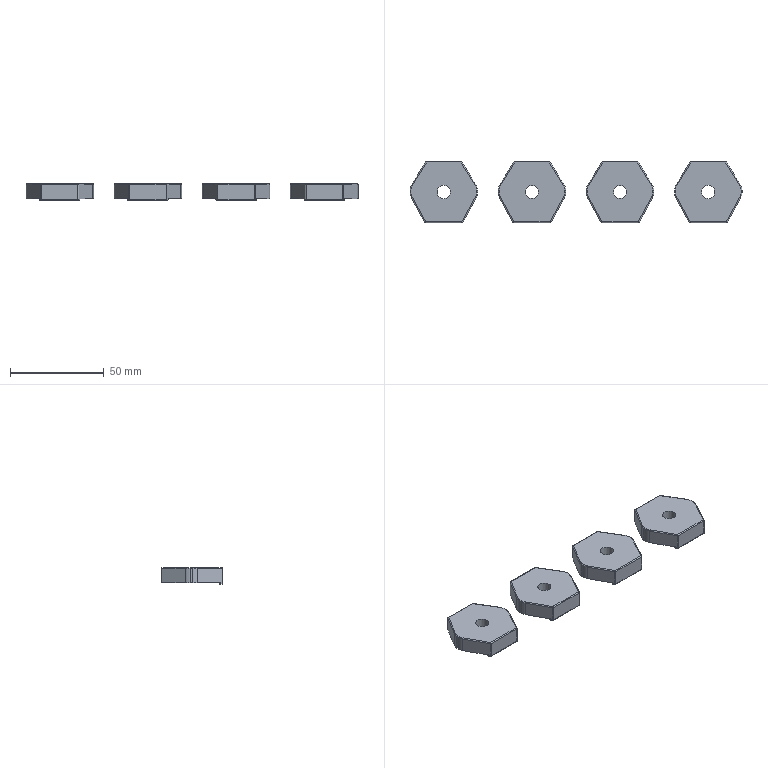Part | 4 solids | 196 faces | box 177 x 33 x 9 mm | volume 29006 mm3 | cylinder 96 | plane 52 | sphere 32 | torus 16 | commonest cylinder face diameters 1 x72 10 x16 3.3 x4 7 x4